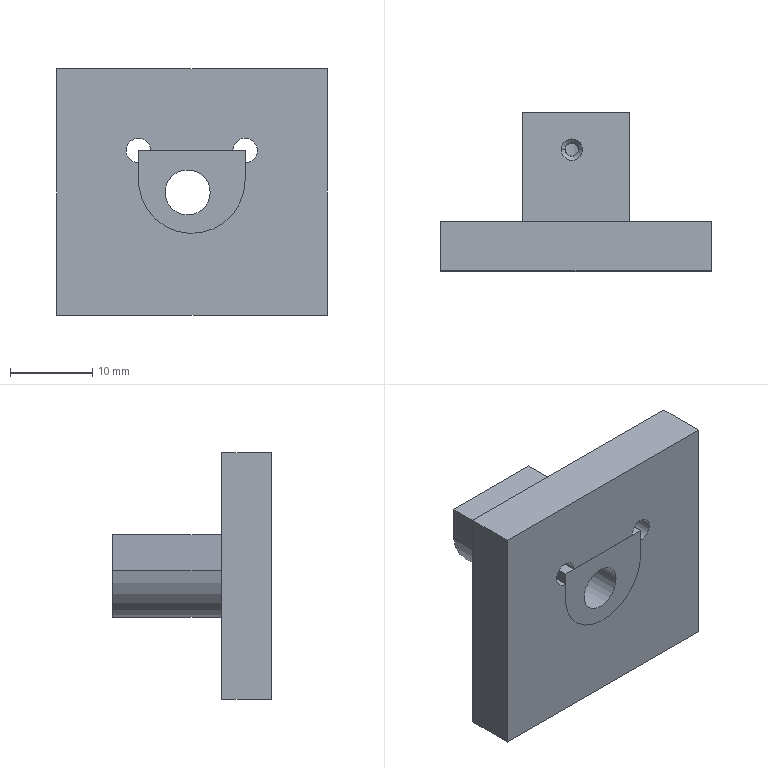NC program | NX | posted with a generic post | part box 32.951 x 19.3 x 30.1 mm
Lines 2828 to 2866 of 2866:
(PLANAR_MILL_COPY , TOOL : D6A45)
N5630 T07 M6
N5632 G54
N5634 G17 G0 G90 X-0.894 Y-0.923 B0. C0. S9500 M3
N5636 G43 Z30. H7
N5638 Z0.5
N5640 G94 G1 Z-1. F1250.
N5642 X-1.266 Y-1.842
N5644 G3 X-0.5 Y-2.2 R1.
N5646 X1.75 Y0.05 R2.25
N5648 X-0.5 Y-2.2 R-2.25
N5650 X0.266 Y-1.842 R1.
N5652 G1 X-0.106 Y-0.923
N5654 Z0.5
N5656 G0 Z30.
(PLANAR_MILL_COPY_COPY , TOOL : D6A45)
N5658 X1.474 Y-7.15
N5660 Z0.5
N5662 G1 Z-1.
N5664 X0.767 Y-6.307
N5666 G3 X0.001 Y-5.95 R1.
N5668 G1 X-6.399
N5670 G2 X-7.399 Y-4.939 R1.
N5672 G1 X-7.351 Y-0.651
N5674 X-7.344 Y-0.539
N5676 G2 X7.4 Y-1.45 R7.4
N5678 G1 Y-4.95
N5680 G2 X6.4 Y-5.95 R1.
N5682 G1 X0.001
N5684 G3 X-0.765 Y-6.307 R1.
N5686 G1 X-1.473 Y-7.15
N5688 Z0.5
N5690 G0 Z30.
N5692 M5
N5694 M2